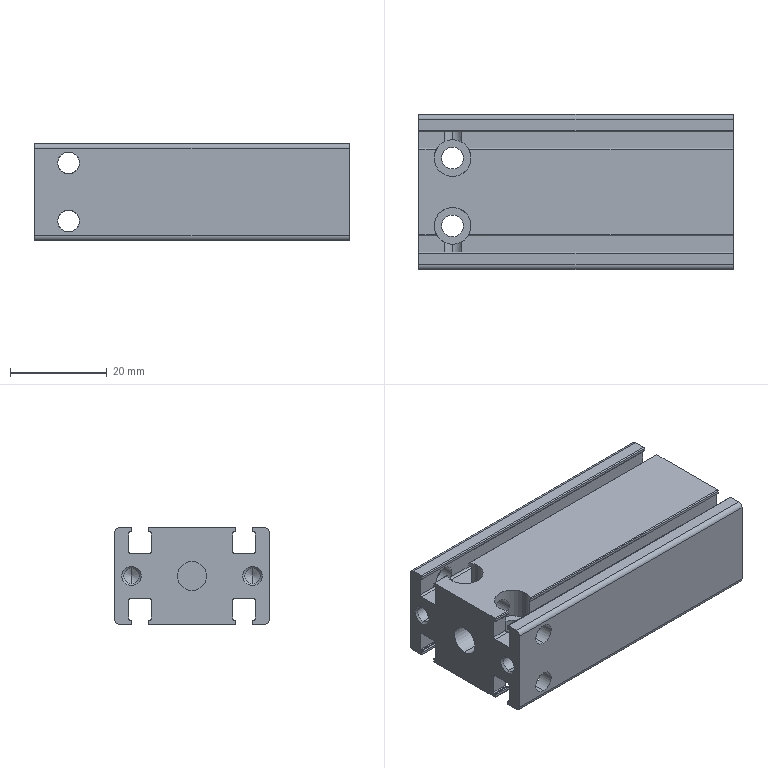Part | SolidWorks | features BaseBody 1 | 1 solid | 181 faces | box 65 x 32 x 20 mm | volume 25563 mm3 | cylinder 98 | plane 63 | cone 20 | commonest cylinder face diameters 0.4 x36 0.8 x16 4.5 x16 3.242 x8 7.6 x8 2 x4